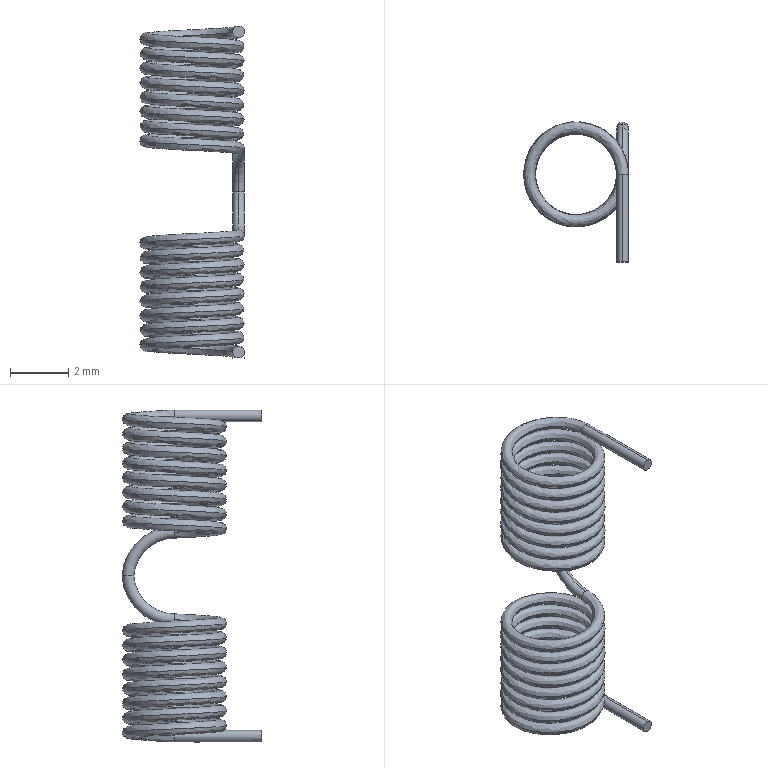Part | SolidWorks | features ICE 4, CompositeCurve 1, Helix 1, MirrorPattern 1, Scale 1, Sweep 1 | 3 solids | 20 faces | box 3.6 x 4.8 x 11.4 mm | volume 21.099 mm3 | torus 6 | cylinder 6 | plane 4 | spline 4 | commonest cylinder face diameters 0.4 x4 0.561 x2